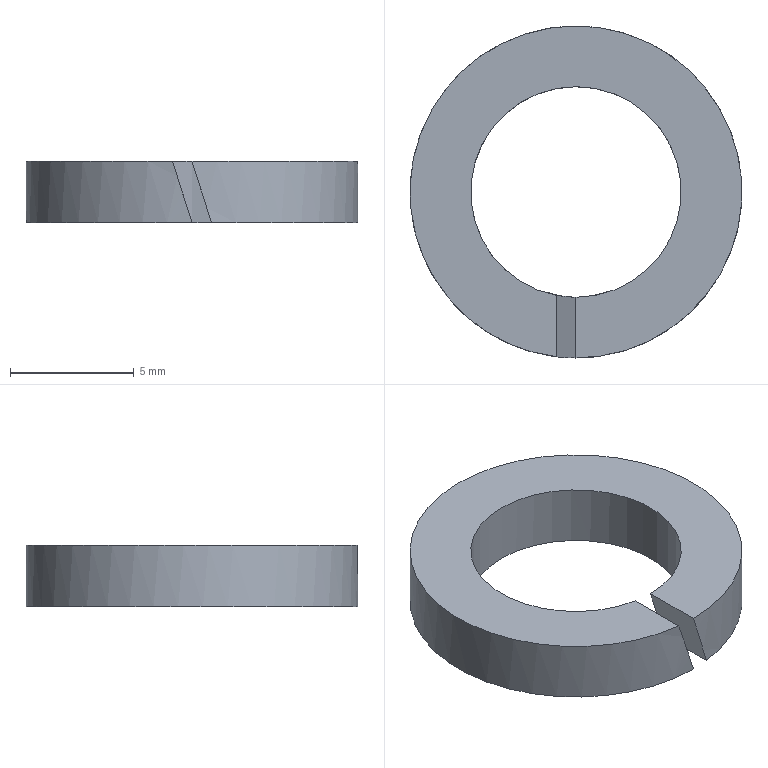Part | STEP file | 1_16 | 1 solid | 6 faces | box 13.4 x 13.4 x 2.5 mm | volume 205.865 mm3 | plane 4 | cylinder 2 | commonest cylinder face diameters 8.5 x1 13.4 x1
STEP:
#1=CARTESIAN_POINT('',(0.,0.,0.));
#2=DIRECTION('',(0.,0.,1.));
#3=DIRECTION('',(1.,0.,0.));
#4=AXIS2_PLACEMENT_3D('',#1,#2,#3);
#5=CARTESIAN_POINT('',(0.7882,-4.176,0.));
#6=VERTEX_POINT('',#5);
#7=CARTESIAN_POINT('',(0.,-4.25,2.5));
#8=VERTEX_POINT('',#7);
#9=CARTESIAN_POINT('',(0.,0.,2.5));
#10=DIRECTION('',(-0.9537,0.,-0.3007));
#11=DIRECTION('',(0.3007,0.,-0.9537));
#12=AXIS2_PLACEMENT_3D('',#9,#10,#11);
#13=ELLIPSE('',#12,14.134,4.25);
#14=CARTESIAN_POINT('',(0.,0.,1.25));
#15=DIRECTION('',(0.,0.,-1.));
#16=DIRECTION('',(1.,0.,0.));
#17=AXIS2_PLACEMENT_3D('',#14,#15,#16);
#18=CYLINDRICAL_SURFACE('',#17,4.25);
#19=CARTESIAN_POINT('',(7.667,1.25));
#20=CARTESIAN_POINT('',(7.854,-1.25));
#21=B_SPLINE_CURVE_WITH_KNOTS('',1,(#19,#20),.UNSPECIFIED.,.F.,.F.,(2,2),(1.384,1.571),.PIECEWISE_BEZIER_KNOTS.);
#22=(GEOMETRIC_REPRESENTATION_CONTEXT(2)PARAMETRIC_REPRESENTATION_CONTEXT()REPRESENTATION_CONTEXT('',''));
#23=DEFINITIONAL_REPRESENTATION('',(#21),#22);
#24=PCURVE('',#18,#23);
#25=CARTESIAN_POINT('',(0.,-4.005,2.5));
#26=DIRECTION('',(0.9537,0.,0.3007));
#27=DIRECTION('',(0.3007,0.,-0.9537));
#28=AXIS2_PLACEMENT_3D('',#25,#26,#27);
#29=PLANE('',#28);
#30=CARTESIAN_POINT('',(14.134,4.005));
#31=CARTESIAN_POINT('',(14.134,-3.356));
#32=CARTESIAN_POINT('',(-7.067,0.3244));
#33=CARTESIAN_POINT('',(-28.267,4.005));
#34=CARTESIAN_POINT('',(-7.067,7.686));
#35=CARTESIAN_POINT('',(14.134,11.366));
#36=CARTESIAN_POINT('',(14.134,4.005));
#37=(BOUNDED_CURVE()B_SPLINE_CURVE(2,(#30,#31,#32,#33,#34,#35,#36),.UNSPECIFIED.,.T.,.F.)B_SPLINE_CURVE_WITH_KNOTS((1,2,2,2,2,1),(-2.094,0.,2.094,4.189,6.283,8.378),.UNSPECIFIED.)CURVE()GEOMETRIC_REPRESENTATION_ITEM()RATIONAL_B_SPLINE_CURVE((1.,0.5,1.,0.5,1.,0.5,1.))REPRESENTATION_ITEM(''));
#38=(GEOMETRIC_REPRESENTATION_CONTEXT(2)PARAMETRIC_REPRESENTATION_CONTEXT()REPRESENTATION_CONTEXT('',''));
#39=DEFINITIONAL_REPRESENTATION('',(#37),#38);
#40=PCURVE('',#29,#39);
#41=SURFACE_CURVE('',#13,(#24,#40),.PCURVE_S1.);
#42=EDGE_CURVE('',#6,#8,#41,.T.);
#43=ORIENTED_EDGE('',*,*,#42,.F.);
#44=CARTESIAN_POINT('',(0.,-4.25,0.));
#45=VERTEX_POINT('',#44);
#46=CARTESIAN_POINT('',(0.,0.,0.));
#47=DIRECTION('',(0.,0.,1.));
#48=DIRECTION('',(1.,0.,0.));
#49=AXIS2_PLACEMENT_3D('',#46,#47,#48);
#50=CIRCLE('',#49,4.25);
#51=CARTESIAN_POINT('',(12.566,1.25));
#52=DIRECTION('',(-1.,0.));
#53=VECTOR('',#52,1.);
#54=LINE('',#51,#53);
#55=(GEOMETRIC_REPRESENTATION_CONTEXT(2)PARAMETRIC_REPRESENTATION_CONTEXT()REPRESENTATION_CONTEXT('',''));
#56=DEFINITIONAL_REPRESENTATION('',(#54),#55);
#57=PCURVE('',#18,#56);
#58=CARTESIAN_POINT('',(5.475,0.,0.));
#59=DIRECTION('',(0.,0.,-1.));
#60=DIRECTION('',(-1.,0.,0.));
#61=AXIS2_PLACEMENT_3D('',#58,#59,#60);
#62=PLANE('',#61);
#63=CARTESIAN_POINT('',(1.225,0.));
#64=CARTESIAN_POINT('',(1.225,7.361));
#65=CARTESIAN_POINT('',(7.6,3.681));
#66=CARTESIAN_POINT('',(13.975,0.));
#67=CARTESIAN_POINT('',(7.6,-3.681));
#68=CARTESIAN_POINT('',(1.225,-7.361));
#69=CARTESIAN_POINT('',(1.225,0.));
#70=(BOUNDED_CURVE()B_SPLINE_CURVE(2,(#63,#64,#65,#66,#67,#68,#69),.UNSPECIFIED.,.T.,.F.)B_SPLINE_CURVE_WITH_KNOTS((1,2,2,2,2,1),(-2.094,0.,2.094,4.189,6.283,8.378),.UNSPECIFIED.)CURVE()GEOMETRIC_REPRESENTATION_ITEM()RATIONAL_B_SPLINE_CURVE((1.,0.5,1.,0.5,1.,0.5,1.))REPRESENTATION_ITEM(''));
#71=(GEOMETRIC_REPRESENTATION_CONTEXT(2)PARAMETRIC_REPRESENTATION_CONTEXT()REPRESENTATION_CONTEXT('',''));
#72=DEFINITIONAL_REPRESENTATION('',(#70),#71);
#73=PCURVE('',#62,#72);
#74=SURFACE_CURVE('',#50,(#57,#73),.PCURVE_S1.);
#75=EDGE_CURVE('',#6,#45,#74,.T.);
#76=ORIENTED_EDGE('',*,*,#75,.T.);
#77=CARTESIAN_POINT('',(-0.7882,-4.176,2.5));
#78=VERTEX_POINT('',#77);
#79=CARTESIAN_POINT('',(0.,0.,0.));
#80=DIRECTION('',(0.9537,0.,0.3007));
#81=DIRECTION('',(0.3007,0.,-0.9537));
#82=AXIS2_PLACEMENT_3D('',#79,#80,#81);
#83=ELLIPSE('',#82,14.134,4.25);
#84=CARTESIAN_POINT('',(1.757,-1.25));
#85=CARTESIAN_POINT('',(1.571,1.25));
#86=B_SPLINE_CURVE_WITH_KNOTS('',1,(#84,#85),.UNSPECIFIED.,.F.,.F.,(2,2),(4.526,4.712),.PIECEWISE_BEZIER_KNOTS.);
#87=(GEOMETRIC_REPRESENTATION_CONTEXT(2)PARAMETRIC_REPRESENTATION_CONTEXT()REPRESENTATION_CONTEXT('',''));
#88=DEFINITIONAL_REPRESENTATION('',(#86),#87);
#89=PCURVE('',#18,#88);
#90=CARTESIAN_POINT('',(0.,-4.005,0.));
#91=DIRECTION('',(-0.9537,0.,-0.3007));
#92=DIRECTION('',(-0.3007,0.,0.9537));
#93=AXIS2_PLACEMENT_3D('',#90,#91,#92);
#94=PLANE('',#93);
#95=CARTESIAN_POINT('',(-14.134,4.005));
#96=CARTESIAN_POINT('',(-14.134,11.366));
#97=CARTESIAN_POINT('',(7.067,7.686));
#98=CARTESIAN_POINT('',(28.267,4.005));
#99=CARTESIAN_POINT('',(7.067,0.3244));
#100=CARTESIAN_POINT('',(-14.134,-3.356));
#101=CARTESIAN_POINT('',(-14.134,4.005));
#102=(BOUNDED_CURVE()B_SPLINE_CURVE(2,(#95,#96,#97,#98,#99,#100,#101),.UNSPECIFIED.,.T.,.F.)B_SPLINE_CURVE_WITH_KNOTS((1,2,2,2,2,1),(-2.094,0.,2.094,4.189,6.283,8.378),.UNSPECIFIED.)CURVE()GEOMETRIC_REPRESENTATION_ITEM()RATIONAL_B_SPLINE_CURVE((1.,0.5,1.,0.5,1.,0.5,1.))REPRESENTATION_ITEM(''));
#103=(GEOMETRIC_REPRESENTATION_CONTEXT(2)PARAMETRIC_REPRESENTATION_CONTEXT()REPRESENTATION_CONTEXT('',''));
#104=DEFINITIONAL_REPRESENTATION('',(#102),#103);
#105=PCURVE('',#94,#104);
#106=SURFACE_CURVE('',#83,(#89,#105),.PCURVE_S1.);
#107=EDGE_CURVE('',#78,#45,#106,.T.);
#108=ORIENTED_EDGE('',*,*,#107,.F.);
#109=CARTESIAN_POINT('',(0.,0.,2.5));
#110=DIRECTION('',(0.,0.,-1.));
#111=DIRECTION('',(1.,0.,0.));
#112=AXIS2_PLACEMENT_3D('',#109,#110,#111);
#113=CIRCLE('',#112,4.25);
#114=CARTESIAN_POINT('',(0.,-1.25));
#115=DIRECTION('',(1.,0.));
#116=VECTOR('',#115,1.);
#117=LINE('',#114,#116);
#118=(GEOMETRIC_REPRESENTATION_CONTEXT(2)PARAMETRIC_REPRESENTATION_CONTEXT()REPRESENTATION_CONTEXT('',''));
#119=DEFINITIONAL_REPRESENTATION('',(#117),#118);
#120=PCURVE('',#18,#119);
#121=CARTESIAN_POINT('',(5.475,0.,2.5));
#122=DIRECTION('',(0.,0.,1.));
#123=DIRECTION('',(1.,0.,0.));
#124=AXIS2_PLACEMENT_3D('',#121,#122,#123);
#125=PLANE('',#124);
#126=CARTESIAN_POINT('',(-1.225,0.));
#127=CARTESIAN_POINT('',(-1.225,-7.361));
#128=CARTESIAN_POINT('',(-7.6,-3.681));
#129=CARTESIAN_POINT('',(-13.975,0.));
#130=CARTESIAN_POINT('',(-7.6,3.681));
#131=CARTESIAN_POINT('',(-1.225,7.361));
#132=CARTESIAN_POINT('',(-1.225,0.));
#133=(BOUNDED_CURVE()B_SPLINE_CURVE(2,(#126,#127,#128,#129,#130,#131,#132),.UNSPECIFIED.,.T.,.F.)B_SPLINE_CURVE_WITH_KNOTS((1,2,2,2,2,1),(-2.094,0.,2.094,4.189,6.283,8.378),.UNSPECIFIED.)CURVE()GEOMETRIC_REPRESENTATION_ITEM()RATIONAL_B_SPLINE_CURVE((1.,0.5,1.,0.5,1.,0.5,1.))REPRESENTATION_ITEM(''));
#134=(GEOMETRIC_REPRESENTATION_CONTEXT(2)PARAMETRIC_REPRESENTATION_CONTEXT()REPRESENTATION_CONTEXT('',''));
#135=DEFINITIONAL_REPRESENTATION('',(#133),#134);
#136=PCURVE('',#125,#135);
#137=SURFACE_CURVE('',#113,(#120,#136),.PCURVE_S1.);
#138=EDGE_CURVE('',#78,#8,#137,.T.);
#139=ORIENTED_EDGE('',*,*,#138,.T.);
#140=EDGE_LOOP('',(#43,#76,#108,#139));
#141=FACE_BOUND('',#140,.F.);
#142=ADVANCED_FACE('',(#141),#18,.F.);
#143=CARTESIAN_POINT('',(0.,-6.7,2.5));
#144=VERTEX_POINT('',#143);
#145=CARTESIAN_POINT('',(0.,-4.25,2.5));
#146=DIRECTION('',(0.,-1.,0.));
#147=VECTOR('',#146,1.);
#148=LINE('',#145,#147);
#149=CARTESIAN_POINT('',(-5.475,-4.25));
#150=DIRECTION('',(0.,-1.));
#151=VECTOR('',#150,1.);
#152=LINE('',#149,#151);
#153=(GEOMETRIC_REPRESENTATION_CONTEXT(2)PARAMETRIC_REPRESENTATION_CONTEXT()REPRESENTATION_CONTEXT('',''));
#154=DEFINITIONAL_REPRESENTATION('',(#152),#153);
#155=PCURVE('',#125,#154);
#156=CARTESIAN_POINT('',(0.,-0.245));
#157=DIRECTION('',(0.,-1.));
#158=VECTOR('',#157,1.);
#159=LINE('',#156,#158);
#160=(GEOMETRIC_REPRESENTATION_CONTEXT(2)PARAMETRIC_REPRESENTATION_CONTEXT()REPRESENTATION_CONTEXT('',''));
#161=DEFINITIONAL_REPRESENTATION('',(#159),#160);
#162=PCURVE('',#29,#161);
#163=SURFACE_CURVE('',#148,(#155,#162),.PCURVE_S1.);
#164=EDGE_CURVE('',#8,#144,#163,.T.);
#165=ORIENTED_EDGE('',*,*,#164,.T.);
#166=CARTESIAN_POINT('',(-0.7882,-6.653,2.5));
#167=VERTEX_POINT('',#166);
#168=CARTESIAN_POINT('',(0.000000004,-0.000000004,2.5));
#169=DIRECTION('',(0.,0.,1.));
#170=DIRECTION('',(1.,0.,0.));
#171=AXIS2_PLACEMENT_3D('',#168,#169,#170);
#172=CIRCLE('',#171,6.7);
#173=CARTESIAN_POINT('',(-5.475,-0.000000004));
#174=DIRECTION('',(1.,0.));
#175=AXIS2_PLACEMENT_2D('',#173,#174);
#176=CIRCLE('',#175,6.7);
#177=(GEOMETRIC_REPRESENTATION_CONTEXT(2)PARAMETRIC_REPRESENTATION_CONTEXT()REPRESENTATION_CONTEXT('',''));
#178=DEFINITIONAL_REPRESENTATION('',(#176),#177);
#179=PCURVE('',#125,#178);
#180=CARTESIAN_POINT('',(0.,0.,1.25));
#181=DIRECTION('',(0.,0.,-1.));
#182=DIRECTION('',(1.,0.,0.));
#183=AXIS2_PLACEMENT_3D('',#180,#181,#182);
#184=CYLINDRICAL_SURFACE('',#183,6.7);
#185=CARTESIAN_POINT('',(12.566,-1.25));
#186=DIRECTION('',(-1.,0.));
#187=VECTOR('',#186,1.);
#188=LINE('',#185,#187);
#189=(GEOMETRIC_REPRESENTATION_CONTEXT(2)PARAMETRIC_REPRESENTATION_CONTEXT()REPRESENTATION_CONTEXT('',''));
#190=DEFINITIONAL_REPRESENTATION('',(#188),#189);
#191=PCURVE('',#184,#190);
#192=SURFACE_CURVE('',#172,(#179,#191),.PCURVE_S1.);
#193=EDGE_CURVE('',#144,#167,#192,.T.);
#194=ORIENTED_EDGE('',*,*,#193,.T.);
#195=CARTESIAN_POINT('',(-0.7882,-6.653,2.5));
#196=DIRECTION('',(0.,1.,0.));
#197=VECTOR('',#196,1.);
#198=LINE('',#195,#197);
#199=CARTESIAN_POINT('',(-6.263,-6.653));
#200=DIRECTION('',(0.,1.));
#201=VECTOR('',#200,1.);
#202=LINE('',#199,#201);
#203=(GEOMETRIC_REPRESENTATION_CONTEXT(2)PARAMETRIC_REPRESENTATION_CONTEXT()REPRESENTATION_CONTEXT('',''));
#204=DEFINITIONAL_REPRESENTATION('',(#202),#203);
#205=PCURVE('',#125,#204);
#206=CARTESIAN_POINT('',(2.621,-2.648));
#207=DIRECTION('',(0.,1.));
#208=VECTOR('',#207,1.);
#209=LINE('',#206,#208);
#210=(GEOMETRIC_REPRESENTATION_CONTEXT(2)PARAMETRIC_REPRESENTATION_CONTEXT()REPRESENTATION_CONTEXT('',''));
#211=DEFINITIONAL_REPRESENTATION('',(#209),#210);
#212=PCURVE('',#94,#211);
#213=SURFACE_CURVE('',#198,(#205,#212),.PCURVE_S1.);
#214=EDGE_CURVE('',#167,#78,#213,.T.);
#215=ORIENTED_EDGE('',*,*,#214,.T.);
#216=ORIENTED_EDGE('',*,*,#138,.T.);
#217=EDGE_LOOP('',(#165,#194,#215,#216));
#218=FACE_BOUND('',#217,.T.);
#219=ADVANCED_FACE('',(#218),#125,.T.);
#220=ORIENTED_EDGE('',*,*,#107,.F.);
#221=ORIENTED_EDGE('',*,*,#214,.F.);
#222=CARTESIAN_POINT('',(0.,-6.7,0.));
#223=VERTEX_POINT('',#222);
#224=CARTESIAN_POINT('',(-0.01466,-0.2484,0.04651));
#225=DIRECTION('',(-0.9537,0.,-0.3007));
#226=DIRECTION('',(0.3007,-0.0007207,-0.9537));
#227=AXIS2_PLACEMENT_3D('',#224,#225,#226);
#228=ELLIPSE('',#227,21.863,6.452);
#229=CARTESIAN_POINT('',(0.04877,3.757));
#230=DIRECTION('',(-1.,-0.0007207));
#231=AXIS2_PLACEMENT_2D('',#229,#230);
#232=ELLIPSE('',#231,21.863,6.452);
#233=(GEOMETRIC_REPRESENTATION_CONTEXT(2)PARAMETRIC_REPRESENTATION_CONTEXT()REPRESENTATION_CONTEXT('',''));
#234=DEFINITIONAL_REPRESENTATION('',(#232),#233);
#235=PCURVE('',#94,#234);
#236=CARTESIAN_POINT('',(1.571,1.25));
#237=CARTESIAN_POINT('',(1.689,-1.25));
#238=B_SPLINE_CURVE_WITH_KNOTS('',1,(#236,#237),.UNSPECIFIED.,.F.,.F.,(2,2),(1.568,1.689),.PIECEWISE_BEZIER_KNOTS.);
#239=(GEOMETRIC_REPRESENTATION_CONTEXT(2)PARAMETRIC_REPRESENTATION_CONTEXT()REPRESENTATION_CONTEXT('',''));
#240=DEFINITIONAL_REPRESENTATION('',(#238),#239);
#241=PCURVE('',#184,#240);
#242=SURFACE_CURVE('',#228,(#235,#241),.PCURVE_S1.);
#243=EDGE_CURVE('',#223,#167,#242,.T.);
#244=ORIENTED_EDGE('',*,*,#243,.F.);
#245=CARTESIAN_POINT('',(0.,-4.25,0.));
#246=DIRECTION('',(0.,-1.,0.));
#247=VECTOR('',#246,1.);
#248=LINE('',#245,#247);
#249=CARTESIAN_POINT('',(0.,-0.245));
#250=DIRECTION('',(0.,-1.));
#251=VECTOR('',#250,1.);
#252=LINE('',#249,#251);
#253=(GEOMETRIC_REPRESENTATION_CONTEXT(2)PARAMETRIC_REPRESENTATION_CONTEXT()REPRESENTATION_CONTEXT('',''));
#254=DEFINITIONAL_REPRESENTATION('',(#252),#253);
#255=PCURVE('',#94,#254);
#256=CARTESIAN_POINT('',(5.475,-4.25));
#257=DIRECTION('',(0.,-1.));
#258=VECTOR('',#257,1.);
#259=LINE('',#256,#258);
#260=(GEOMETRIC_REPRESENTATION_CONTEXT(2)PARAMETRIC_REPRESENTATION_CONTEXT()REPRESENTATION_CONTEXT('',''));
#261=DEFINITIONAL_REPRESENTATION('',(#259),#260);
#262=PCURVE('',#62,#261);
#263=SURFACE_CURVE('',#248,(#255,#262),.PCURVE_S1.);
#264=EDGE_CURVE('',#45,#223,#263,.T.);
#265=ORIENTED_EDGE('',*,*,#264,.F.);
#266=EDGE_LOOP('',(#220,#221,#244,#265));
#267=FACE_BOUND('',#266,.T.);
#268=ADVANCED_FACE('',(#267),#94,.F.);
#269=CARTESIAN_POINT('',(0.7882,-6.653,0.));
#270=VERTEX_POINT('',#269);
#271=CARTESIAN_POINT('',(0.7882,-6.653,0.));
#272=DIRECTION('',(0.,1.,0.));
#273=VECTOR('',#272,1.);
#274=LINE('',#271,#273);
#275=CARTESIAN_POINT('',(4.687,-6.653));
#276=DIRECTION('',(0.,1.));
#277=VECTOR('',#276,1.);
#278=LINE('',#275,#277);
#279=(GEOMETRIC_REPRESENTATION_CONTEXT(2)PARAMETRIC_REPRESENTATION_CONTEXT()REPRESENTATION_CONTEXT('',''));
#280=DEFINITIONAL_REPRESENTATION('',(#278),#279);
#281=PCURVE('',#62,#280);
#282=CARTESIAN_POINT('',(2.621,-2.648));
#283=DIRECTION('',(0.,1.));
#284=VECTOR('',#283,1.);
#285=LINE('',#282,#284);
#286=(GEOMETRIC_REPRESENTATION_CONTEXT(2)PARAMETRIC_REPRESENTATION_CONTEXT()REPRESENTATION_CONTEXT('',''));
#287=DEFINITIONAL_REPRESENTATION('',(#285),#286);
#288=PCURVE('',#29,#287);
#289=SURFACE_CURVE('',#274,(#281,#288),.PCURVE_S1.);
#290=EDGE_CURVE('',#270,#6,#289,.T.);
#291=ORIENTED_EDGE('',*,*,#290,.T.);
#292=ORIENTED_EDGE('',*,*,#75,.T.);
#293=ORIENTED_EDGE('',*,*,#264,.T.);
#294=CARTESIAN_POINT('',(0.,0.,0.));
#295=DIRECTION('',(0.,0.,1.));
#296=DIRECTION('',(0.,-1.,0.));
#297=AXIS2_PLACEMENT_3D('',#294,#295,#296);
#298=CIRCLE('',#297,6.7);
#299=CARTESIAN_POINT('',(5.475,-6.7));
#300=CARTESIAN_POINT('',(-6.13,-6.7));
#301=CARTESIAN_POINT('',(-0.3274,3.35));
#302=CARTESIAN_POINT('',(5.475,13.4));
#303=CARTESIAN_POINT('',(11.277,3.35));
#304=CARTESIAN_POINT('',(17.08,-6.7));
#305=CARTESIAN_POINT('',(5.475,-6.7));
#306=(BOUNDED_CURVE()B_SPLINE_CURVE(2,(#299,#300,#301,#302,#303,#304,#305),.UNSPECIFIED.,.T.,.F.)B_SPLINE_CURVE_WITH_KNOTS((1,2,2,2,2,1),(-2.094,0.,2.094,4.189,6.283,8.378),.UNSPECIFIED.)CURVE()GEOMETRIC_REPRESENTATION_ITEM()RATIONAL_B_SPLINE_CURVE((1.,0.5,1.,0.5,1.,0.5,1.))REPRESENTATION_ITEM(''));
#307=(GEOMETRIC_REPRESENTATION_CONTEXT(2)PARAMETRIC_REPRESENTATION_CONTEXT()REPRESENTATION_CONTEXT('',''));
#308=DEFINITIONAL_REPRESENTATION('',(#306),#307);
#309=PCURVE('',#62,#308);
#310=CARTESIAN_POINT('',(7.854,1.25));
#311=DIRECTION('',(-1.,0.));
#312=VECTOR('',#311,1.);
#313=LINE('',#310,#312);
#314=(GEOMETRIC_REPRESENTATION_CONTEXT(2)PARAMETRIC_REPRESENTATION_CONTEXT()REPRESENTATION_CONTEXT('',''));
#315=DEFINITIONAL_REPRESENTATION('',(#313),#314);
#316=PCURVE('',#184,#315);
#317=SURFACE_CURVE('',#298,(#309,#316),.PCURVE_S1.);
#318=EDGE_CURVE('',#270,#223,#317,.T.);
#319=ORIENTED_EDGE('',*,*,#318,.F.);
#320=EDGE_LOOP('',(#291,#292,#293,#319));
#321=FACE_BOUND('',#320,.T.);
#322=ADVANCED_FACE('',(#321),#62,.T.);
#323=ORIENTED_EDGE('',*,*,#42,.F.);
#324=ORIENTED_EDGE('',*,*,#290,.F.);
#325=CARTESIAN_POINT('',(0.01466,-0.2484,2.453));
#326=DIRECTION('',(0.9537,0.,0.3007));
#327=DIRECTION('',(0.3007,0.0007207,-0.9537));
#328=AXIS2_PLACEMENT_3D('',#325,#326,#327);
#329=ELLIPSE('',#328,21.863,6.452);
#330=CARTESIAN_POINT('',(0.04877,3.757));
#331=DIRECTION('',(1.,0.0007207));
#332=AXIS2_PLACEMENT_2D('',#330,#331);
#333=ELLIPSE('',#332,21.863,6.452);
#334=(GEOMETRIC_REPRESENTATION_CONTEXT(2)PARAMETRIC_REPRESENTATION_CONTEXT()REPRESENTATION_CONTEXT('',''));
#335=DEFINITIONAL_REPRESENTATION('',(#333),#334);
#336=PCURVE('',#29,#335);
#337=CARTESIAN_POINT('',(7.854,-1.25));
#338=CARTESIAN_POINT('',(7.736,1.25));
#339=B_SPLINE_CURVE_WITH_KNOTS('',1,(#337,#338),.UNSPECIFIED.,.F.,.F.,(2,2),(4.71,4.83),.PIECEWISE_BEZIER_KNOTS.);
#340=(GEOMETRIC_REPRESENTATION_CONTEXT(2)PARAMETRIC_REPRESENTATION_CONTEXT()REPRESENTATION_CONTEXT('',''));
#341=DEFINITIONAL_REPRESENTATION('',(#339),#340);
#342=PCURVE('',#184,#341);
#343=SURFACE_CURVE('',#329,(#336,#342),.PCURVE_S1.);
#344=EDGE_CURVE('',#144,#270,#343,.T.);
#345=ORIENTED_EDGE('',*,*,#344,.F.);
#346=ORIENTED_EDGE('',*,*,#164,.F.);
#347=EDGE_LOOP('',(#323,#324,#345,#346));
#348=FACE_BOUND('',#347,.T.);
#349=ADVANCED_FACE('',(#348),#29,.F.);
#350=ORIENTED_EDGE('',*,*,#193,.F.);
#351=ORIENTED_EDGE('',*,*,#344,.T.);
#352=ORIENTED_EDGE('',*,*,#318,.T.);
#353=ORIENTED_EDGE('',*,*,#243,.T.);
#354=EDGE_LOOP('',(#350,#351,#352,#353));
#355=FACE_BOUND('',#354,.T.);
#356=ADVANCED_FACE('',(#355),#184,.T.);
#357=CLOSED_SHELL('',(#142,#219,#268,#322,#349,#356));
#358=MANIFOLD_SOLID_BREP('',#357);
#359=(LENGTH_UNIT()NAMED_UNIT(*)SI_UNIT(.MILLI.,.METRE.));
#360=UNCERTAINTY_MEASURE_WITH_UNIT(LENGTH_MEASURE(0.002),#359,'','');
#361=(NAMED_UNIT(*)PLANE_ANGLE_UNIT()SI_UNIT($,.RADIAN.));
#362=(NAMED_UNIT(*)SI_UNIT($,.STERADIAN.)SOLID_ANGLE_UNIT());
#363=(GEOMETRIC_REPRESENTATION_CONTEXT(3)GLOBAL_UNCERTAINTY_ASSIGNED_CONTEXT((#360))GLOBAL_UNIT_ASSIGNED_CONTEXT((#359,#361,#362))REPRESENTATION_CONTEXT('',''));
#364=ADVANCED_BREP_SHAPE_REPRESENTATION('',(#4,#358),#363);